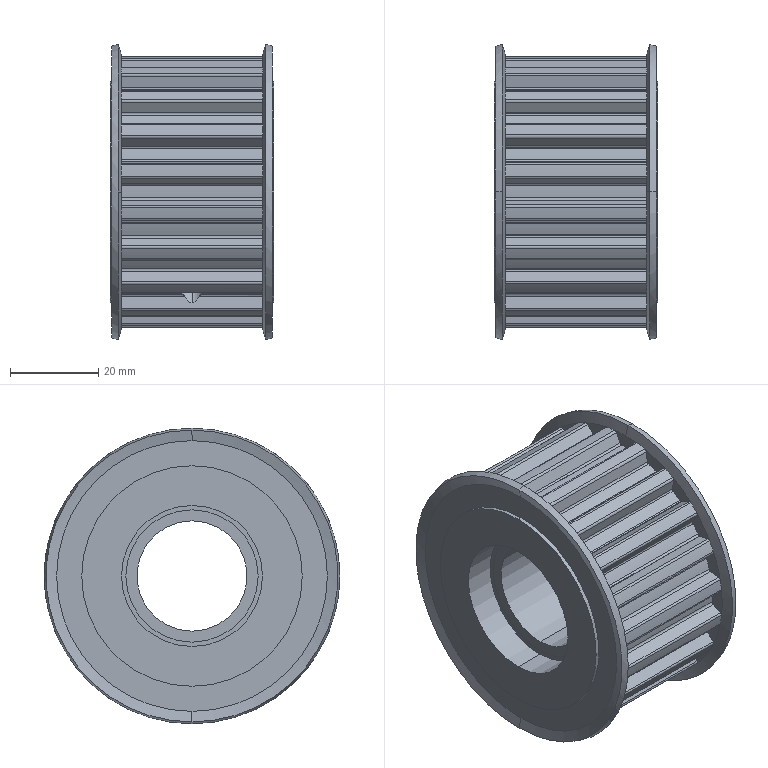Part | SolidWorks | features ICE 3, BaseBody 2 | 3 solids | 267 faces | box 37 x 67 x 67 mm | volume 77744 mm3 | cylinder 163 | plane 88 | cone 12 | spline 4 | commonest cylinder face diameters 1 x50 1.2 x50 55.4 x23 61.8 x20 30 x6 4.917 x4